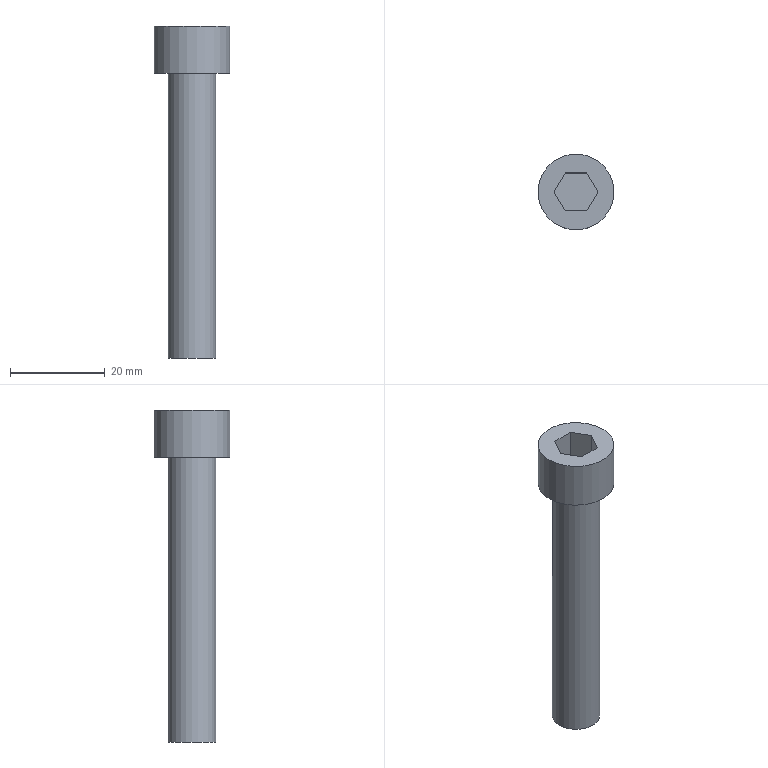Part | STEP file | lll_id626_x_t | 1 solid | 12 faces | box 16 x 16 x 70 mm | volume 6357 mm3 | plane 10 | cylinder 2 | commonest cylinder face diameters 10 x1 16 x1
STEP:
#1=CARTESIAN_POINT('',(-89.,-77.,153.5));
#2=VERTEX_POINT('',#1);
#3=CARTESIAN_POINT('',(-97.,-77.,153.5));
#4=DIRECTION('',(0.,0.,1.));
#5=DIRECTION('',(1.,0.,0.));
#6=AXIS2_PLACEMENT_3D('',#3,#4,#5);
#7=CIRCLE('',#6,8.);
#8=EDGE_CURVE('',#2,#2,#7,.T.);
#9=ORIENTED_EDGE('',*,*,#8,.T.);
#10=EDGE_LOOP('',(#9));
#11=FACE_BOUND('',#10,.T.);
#12=CARTESIAN_POINT('',(-99.309,-73.,153.5));
#13=VERTEX_POINT('',#12);
#14=CARTESIAN_POINT('',(-94.691,-73.,153.5));
#15=VERTEX_POINT('',#14);
#16=CARTESIAN_POINT('',(-99.309,-73.,153.5));
#17=DIRECTION('',(1.,0.,0.));
#18=VECTOR('',#17,1.);
#19=LINE('',#16,#18);
#20=EDGE_CURVE('',#13,#15,#19,.T.);
#21=ORIENTED_EDGE('',*,*,#20,.T.);
#22=CARTESIAN_POINT('',(-92.381,-77.,153.5));
#23=VERTEX_POINT('',#22);
#24=CARTESIAN_POINT('',(-94.691,-73.,153.5));
#25=DIRECTION('',(0.5,-0.866,0.));
#26=VECTOR('',#25,1.);
#27=LINE('',#24,#26);
#28=EDGE_CURVE('',#15,#23,#27,.T.);
#29=ORIENTED_EDGE('',*,*,#28,.T.);
#30=CARTESIAN_POINT('',(-94.691,-81.,153.5));
#31=VERTEX_POINT('',#30);
#32=CARTESIAN_POINT('',(-92.381,-77.,153.5));
#33=DIRECTION('',(-0.5,-0.866,0.));
#34=VECTOR('',#33,1.);
#35=LINE('',#32,#34);
#36=EDGE_CURVE('',#23,#31,#35,.T.);
#37=ORIENTED_EDGE('',*,*,#36,.T.);
#38=CARTESIAN_POINT('',(-99.309,-81.,153.5));
#39=VERTEX_POINT('',#38);
#40=CARTESIAN_POINT('',(-94.691,-81.,153.5));
#41=DIRECTION('',(-1.,0.,0.));
#42=VECTOR('',#41,1.);
#43=LINE('',#40,#42);
#44=EDGE_CURVE('',#31,#39,#43,.T.);
#45=ORIENTED_EDGE('',*,*,#44,.T.);
#46=CARTESIAN_POINT('',(-101.619,-77.,153.5));
#47=VERTEX_POINT('',#46);
#48=CARTESIAN_POINT('',(-99.309,-81.,153.5));
#49=DIRECTION('',(-0.5,0.866,0.));
#50=VECTOR('',#49,1.);
#51=LINE('',#48,#50);
#52=EDGE_CURVE('',#39,#47,#51,.T.);
#53=ORIENTED_EDGE('',*,*,#52,.T.);
#54=CARTESIAN_POINT('',(-101.619,-77.,153.5));
#55=DIRECTION('',(0.5,0.866,0.));
#56=VECTOR('',#55,1.);
#57=LINE('',#54,#56);
#58=EDGE_CURVE('',#47,#13,#57,.T.);
#59=ORIENTED_EDGE('',*,*,#58,.T.);
#60=EDGE_LOOP('',(#21,#29,#37,#45,#53,#59));
#61=FACE_BOUND('',#60,.T.);
#62=CARTESIAN_POINT('',(-89.,-77.,153.5));
#63=DIRECTION('',(0.,0.,-1.));
#64=DIRECTION('',(-1.,0.,0.));
#65=AXIS2_PLACEMENT_3D('',#62,#63,#64);
#66=PLANE('',#65);
#67=ADVANCED_FACE('',(#11,#61),#66,.F.);
#68=ORIENTED_EDGE('',*,*,#8,.F.);
#69=EDGE_LOOP('',(#68));
#70=FACE_BOUND('',#69,.T.);
#71=CARTESIAN_POINT('',(-89.,-77.,143.5));
#72=VERTEX_POINT('',#71);
#73=CARTESIAN_POINT('',(-97.,-77.,143.5));
#74=DIRECTION('',(0.,0.,1.));
#75=DIRECTION('',(1.,0.,0.));
#76=AXIS2_PLACEMENT_3D('',#73,#74,#75);
#77=CIRCLE('',#76,8.);
#78=EDGE_CURVE('',#72,#72,#77,.T.);
#79=ORIENTED_EDGE('',*,*,#78,.T.);
#80=EDGE_LOOP('',(#79));
#81=FACE_BOUND('',#80,.T.);
#82=CARTESIAN_POINT('',(-97.,-77.,144.6));
#83=DIRECTION('',(0.,0.,1.));
#84=DIRECTION('',(1.,0.,0.));
#85=AXIS2_PLACEMENT_3D('',#82,#83,#84);
#86=CYLINDRICAL_SURFACE('',#85,8.);
#87=ADVANCED_FACE('',(#70,#81),#86,.T.);
#88=ORIENTED_EDGE('',*,*,#78,.F.);
#89=EDGE_LOOP('',(#88));
#90=FACE_BOUND('',#89,.T.);
#91=CARTESIAN_POINT('',(-92.,-77.,143.5));
#92=VERTEX_POINT('',#91);
#93=CARTESIAN_POINT('',(-97.,-77.,143.5));
#94=DIRECTION('',(0.,0.,1.));
#95=DIRECTION('',(1.,0.,0.));
#96=AXIS2_PLACEMENT_3D('',#93,#94,#95);
#97=CIRCLE('',#96,5.);
#98=EDGE_CURVE('',#92,#92,#97,.T.);
#99=ORIENTED_EDGE('',*,*,#98,.T.);
#100=EDGE_LOOP('',(#99));
#101=FACE_BOUND('',#100,.T.);
#102=CARTESIAN_POINT('',(-92.,-77.,143.5));
#103=DIRECTION('',(0.,0.,1.));
#104=DIRECTION('',(1.,0.,0.));
#105=AXIS2_PLACEMENT_3D('',#102,#103,#104);
#106=PLANE('',#105);
#107=ADVANCED_FACE('',(#90,#101),#106,.F.);
#108=ORIENTED_EDGE('',*,*,#98,.F.);
#109=EDGE_LOOP('',(#108));
#110=FACE_BOUND('',#109,.T.);
#111=CARTESIAN_POINT('',(-92.,-77.,83.5));
#112=VERTEX_POINT('',#111);
#113=CARTESIAN_POINT('',(-97.,-77.,83.5));
#114=DIRECTION('',(0.,0.,1.));
#115=DIRECTION('',(1.,0.,0.));
#116=AXIS2_PLACEMENT_3D('',#113,#114,#115);
#117=CIRCLE('',#116,5.);
#118=EDGE_CURVE('',#112,#112,#117,.T.);
#119=ORIENTED_EDGE('',*,*,#118,.T.);
#120=EDGE_LOOP('',(#119));
#121=FACE_BOUND('',#120,.T.);
#122=CARTESIAN_POINT('',(-97.,-77.,144.6));
#123=DIRECTION('',(0.,0.,1.));
#124=DIRECTION('',(1.,0.,0.));
#125=AXIS2_PLACEMENT_3D('',#122,#123,#124);
#126=CYLINDRICAL_SURFACE('',#125,5.);
#127=ADVANCED_FACE('',(#110,#121),#126,.T.);
#128=ORIENTED_EDGE('',*,*,#118,.F.);
#129=EDGE_LOOP('',(#128));
#130=FACE_OUTER_BOUND('',#129,.T.);
#131=CARTESIAN_POINT('',(-97.,-77.,83.5));
#132=DIRECTION('',(0.,0.,1.));
#133=DIRECTION('',(1.,0.,0.));
#134=AXIS2_PLACEMENT_3D('',#131,#132,#133);
#135=PLANE('',#134);
#136=ADVANCED_FACE('',(#130),#135,.F.);
#137=ORIENTED_EDGE('',*,*,#20,.F.);
#138=CARTESIAN_POINT('',(-99.309,-73.,146.9));
#139=VERTEX_POINT('',#138);
#140=CARTESIAN_POINT('',(-99.309,-73.,146.9));
#141=DIRECTION('',(0.,0.,-1.));
#142=VECTOR('',#141,1.);
#143=LINE('',#140,#142);
#144=EDGE_CURVE('',#13,#139,#143,.T.);
#145=ORIENTED_EDGE('',*,*,#144,.T.);
#146=CARTESIAN_POINT('',(-94.691,-73.,146.9));
#147=VERTEX_POINT('',#146);
#148=CARTESIAN_POINT('',(-99.309,-73.,146.9));
#149=DIRECTION('',(-1.,0.,0.));
#150=VECTOR('',#149,1.);
#151=LINE('',#148,#150);
#152=EDGE_CURVE('',#147,#139,#151,.T.);
#153=ORIENTED_EDGE('',*,*,#152,.F.);
#154=CARTESIAN_POINT('',(-94.691,-73.,146.9));
#155=DIRECTION('',(0.,0.,-1.));
#156=VECTOR('',#155,1.);
#157=LINE('',#154,#156);
#158=EDGE_CURVE('',#15,#147,#157,.T.);
#159=ORIENTED_EDGE('',*,*,#158,.F.);
#160=EDGE_LOOP('',(#137,#145,#153,#159));
#161=FACE_OUTER_BOUND('',#160,.T.);
#162=CARTESIAN_POINT('',(-99.309,-73.,146.9));
#163=DIRECTION('',(0.,-1.,0.));
#164=DIRECTION('',(1.,0.,0.));
#165=AXIS2_PLACEMENT_3D('',#162,#163,#164);
#166=PLANE('',#165);
#167=ADVANCED_FACE('',(#161),#166,.T.);
#168=ORIENTED_EDGE('',*,*,#28,.F.);
#169=ORIENTED_EDGE('',*,*,#158,.T.);
#170=CARTESIAN_POINT('',(-92.381,-77.,146.9));
#171=VERTEX_POINT('',#170);
#172=CARTESIAN_POINT('',(-94.691,-73.,146.9));
#173=DIRECTION('',(-0.5,0.866,0.));
#174=VECTOR('',#173,1.);
#175=LINE('',#172,#174);
#176=EDGE_CURVE('',#171,#147,#175,.T.);
#177=ORIENTED_EDGE('',*,*,#176,.F.);
#178=CARTESIAN_POINT('',(-92.381,-77.,146.9));
#179=DIRECTION('',(0.,0.,-1.));
#180=VECTOR('',#179,1.);
#181=LINE('',#178,#180);
#182=EDGE_CURVE('',#23,#171,#181,.T.);
#183=ORIENTED_EDGE('',*,*,#182,.F.);
#184=EDGE_LOOP('',(#168,#169,#177,#183));
#185=FACE_OUTER_BOUND('',#184,.T.);
#186=CARTESIAN_POINT('',(-94.691,-73.,146.9));
#187=DIRECTION('',(-0.866,-0.5,0.));
#188=DIRECTION('',(0.5,-0.866,0.));
#189=AXIS2_PLACEMENT_3D('',#186,#187,#188);
#190=PLANE('',#189);
#191=ADVANCED_FACE('',(#185),#190,.T.);
#192=ORIENTED_EDGE('',*,*,#36,.F.);
#193=ORIENTED_EDGE('',*,*,#182,.T.);
#194=CARTESIAN_POINT('',(-94.691,-81.,146.9));
#195=VERTEX_POINT('',#194);
#196=CARTESIAN_POINT('',(-92.381,-77.,146.9));
#197=DIRECTION('',(0.5,0.866,0.));
#198=VECTOR('',#197,1.);
#199=LINE('',#196,#198);
#200=EDGE_CURVE('',#195,#171,#199,.T.);
#201=ORIENTED_EDGE('',*,*,#200,.F.);
#202=CARTESIAN_POINT('',(-94.691,-81.,146.9));
#203=DIRECTION('',(0.,0.,-1.));
#204=VECTOR('',#203,1.);
#205=LINE('',#202,#204);
#206=EDGE_CURVE('',#31,#195,#205,.T.);
#207=ORIENTED_EDGE('',*,*,#206,.F.);
#208=EDGE_LOOP('',(#192,#193,#201,#207));
#209=FACE_OUTER_BOUND('',#208,.T.);
#210=CARTESIAN_POINT('',(-92.381,-77.,146.9));
#211=DIRECTION('',(-0.866,0.5,0.));
#212=DIRECTION('',(-0.5,-0.866,0.));
#213=AXIS2_PLACEMENT_3D('',#210,#211,#212);
#214=PLANE('',#213);
#215=ADVANCED_FACE('',(#209),#214,.T.);
#216=ORIENTED_EDGE('',*,*,#44,.F.);
#217=ORIENTED_EDGE('',*,*,#206,.T.);
#218=CARTESIAN_POINT('',(-99.309,-81.,146.9));
#219=VERTEX_POINT('',#218);
#220=CARTESIAN_POINT('',(-94.691,-81.,146.9));
#221=DIRECTION('',(1.,0.,0.));
#222=VECTOR('',#221,1.);
#223=LINE('',#220,#222);
#224=EDGE_CURVE('',#219,#195,#223,.T.);
#225=ORIENTED_EDGE('',*,*,#224,.F.);
#226=CARTESIAN_POINT('',(-99.309,-81.,146.9));
#227=DIRECTION('',(0.,0.,-1.));
#228=VECTOR('',#227,1.);
#229=LINE('',#226,#228);
#230=EDGE_CURVE('',#39,#219,#229,.T.);
#231=ORIENTED_EDGE('',*,*,#230,.F.);
#232=EDGE_LOOP('',(#216,#217,#225,#231));
#233=FACE_OUTER_BOUND('',#232,.T.);
#234=CARTESIAN_POINT('',(-94.691,-81.,146.9));
#235=DIRECTION('',(0.,1.,0.));
#236=DIRECTION('',(0.,0.,1.));
#237=AXIS2_PLACEMENT_3D('',#234,#235,#236);
#238=PLANE('',#237);
#239=ADVANCED_FACE('',(#233),#238,.T.);
#240=ORIENTED_EDGE('',*,*,#52,.F.);
#241=ORIENTED_EDGE('',*,*,#230,.T.);
#242=CARTESIAN_POINT('',(-101.619,-77.,146.9));
#243=VERTEX_POINT('',#242);
#244=CARTESIAN_POINT('',(-99.309,-81.,146.9));
#245=DIRECTION('',(0.5,-0.866,0.));
#246=VECTOR('',#245,1.);
#247=LINE('',#244,#246);
#248=EDGE_CURVE('',#243,#219,#247,.T.);
#249=ORIENTED_EDGE('',*,*,#248,.F.);
#250=CARTESIAN_POINT('',(-101.619,-77.,146.9));
#251=DIRECTION('',(0.,0.,-1.));
#252=VECTOR('',#251,1.);
#253=LINE('',#250,#252);
#254=EDGE_CURVE('',#47,#243,#253,.T.);
#255=ORIENTED_EDGE('',*,*,#254,.F.);
#256=EDGE_LOOP('',(#240,#241,#249,#255));
#257=FACE_OUTER_BOUND('',#256,.T.);
#258=CARTESIAN_POINT('',(-99.309,-81.,146.9));
#259=DIRECTION('',(0.866,0.5,0.));
#260=DIRECTION('',(-0.5,0.866,0.));
#261=AXIS2_PLACEMENT_3D('',#258,#259,#260);
#262=PLANE('',#261);
#263=ADVANCED_FACE('',(#257),#262,.T.);
#264=ORIENTED_EDGE('',*,*,#58,.F.);
#265=ORIENTED_EDGE('',*,*,#254,.T.);
#266=CARTESIAN_POINT('',(-101.619,-77.,146.9));
#267=DIRECTION('',(-0.5,-0.866,0.));
#268=VECTOR('',#267,1.);
#269=LINE('',#266,#268);
#270=EDGE_CURVE('',#139,#243,#269,.T.);
#271=ORIENTED_EDGE('',*,*,#270,.F.);
#272=ORIENTED_EDGE('',*,*,#144,.F.);
#273=EDGE_LOOP('',(#264,#265,#271,#272));
#274=FACE_OUTER_BOUND('',#273,.T.);
#275=CARTESIAN_POINT('',(-101.619,-77.,146.9));
#276=DIRECTION('',(0.866,-0.5,0.));
#277=DIRECTION('',(0.5,0.866,0.));
#278=AXIS2_PLACEMENT_3D('',#275,#276,#277);
#279=PLANE('',#278);
#280=ADVANCED_FACE('',(#274),#279,.T.);
#281=ORIENTED_EDGE('',*,*,#152,.T.);
#282=ORIENTED_EDGE('',*,*,#270,.T.);
#283=ORIENTED_EDGE('',*,*,#248,.T.);
#284=ORIENTED_EDGE('',*,*,#224,.T.);
#285=ORIENTED_EDGE('',*,*,#200,.T.);
#286=ORIENTED_EDGE('',*,*,#176,.T.);
#287=EDGE_LOOP('',(#281,#282,#283,#284,#285,#286));
#288=FACE_OUTER_BOUND('',#287,.T.);
#289=CARTESIAN_POINT('',(-97.,-77.,146.9));
#290=DIRECTION('',(0.,0.,-1.));
#291=DIRECTION('',(-1.,0.,0.));
#292=AXIS2_PLACEMENT_3D('',#289,#290,#291);
#293=PLANE('',#292);
#294=ADVANCED_FACE('',(#288),#293,.F.);
#295=CLOSED_SHELL('',(#67,#87,#107,#127,#136,#167,#191,#215,#239,#263,#280,#294));
#296=MANIFOLD_SOLID_BREP('',#295);
#297=(LENGTH_UNIT()NAMED_UNIT(*)SI_UNIT(.MILLI.,.METRE.));
#298=UNCERTAINTY_MEASURE_WITH_UNIT(LENGTH_MEASURE(0.00002),#297,'','');
#299=(NAMED_UNIT(*)PLANE_ANGLE_UNIT()SI_UNIT($,.RADIAN.));
#300=PLANE_ANGLE_MEASURE_WITH_UNIT(PLANE_ANGLE_MEASURE(0.01745),#299);
#301=DIMENSIONAL_EXPONENTS(0.,0.,0.,0.,0.,0.,0.);
#302=(CONVERSION_BASED_UNIT('DEGREE',#300)NAMED_UNIT(#301)PLANE_ANGLE_UNIT());
#303=(NAMED_UNIT(*)SI_UNIT($,.STERADIAN.)SOLID_ANGLE_UNIT());
#304=(GEOMETRIC_REPRESENTATION_CONTEXT(3)GLOBAL_UNCERTAINTY_ASSIGNED_CONTEXT((#298))GLOBAL_UNIT_ASSIGNED_CONTEXT((#297,#302,#303))REPRESENTATION_CONTEXT('',''));
#305=ADVANCED_BREP_SHAPE_REPRESENTATION('',(#296),#304);